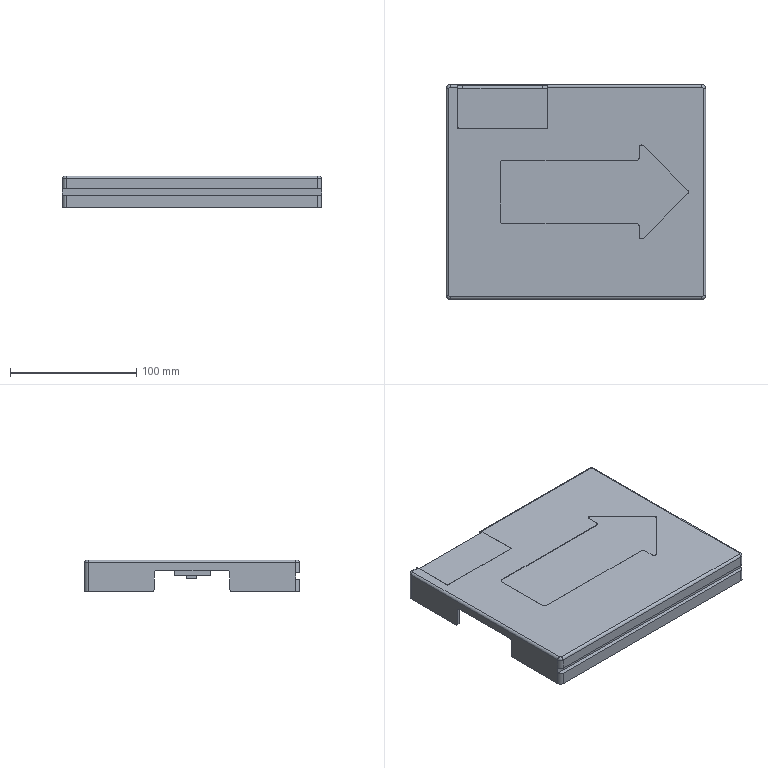NC program | NX | posted with a generic post | part box 205 x 170 x 25 mm
Lines 6527 to 7366 of 17262:
(CAVITY_MILL_1_COPY , TOOL : D4)
N13040 T17 M6
N13042 G54
N13044 G17 G0 G90 X-97.7 Y-73.808 B0. C0. S9500 M3
N13046 G43 Z30. H17
N13048 Z-0.4
N13050 G94 G1 X-98. Y-73.981 F1000.
N13052 G3 X-98.5 Y-74.847 R1.
N13054 G1 Y-76.999 F1600.
N13056 G3 X-97.494 Y-78. R1.
N13058 G1 X-95.347
N13060 G3 X-94.481 Y-77.5 R1.
N13062 G1 X-94.308 Y-77.2
N13064 G0 X-97.7 Y-73.808 Z-0.8
N13066 G1 X-98. Y-73.981 F1000.
N13068 G3 X-98.5 Y-74.847 R1.
N13070 G1 Y-76.999 F1600.
N13072 G3 X-97.494 Y-78. R1.
N13074 G1 X-95.347
N13076 G3 X-94.481 Y-77.5 R1.
N13078 G1 X-94.308 Y-77.2
N13080 G0 X-97.7 Y-73.808 Z-1.2
N13082 G1 X-98. Y-73.981 F1000.
N13084 G3 X-98.5 Y-74.847 R1.
N13086 G1 Y-76.999 F1600.
N13088 G3 X-97.494 Y-78. R1.
N13090 G1 X-95.347
N13092 G3 X-94.481 Y-77.5 R1.
N13094 G1 X-94.308 Y-77.2
N13096 G0 X-97.7 Y-73.808 Z-1.6
N13098 G1 X-98. Y-73.981 F1000.
N13100 G3 X-98.5 Y-74.847 R1.
N13102 G1 Y-76.999 F1600.
N13104 G3 X-97.494 Y-78. R1.
N13106 G1 X-95.347
N13108 G3 X-94.481 Y-77.5 R1.
N13110 G1 X-94.308 Y-77.2
N13112 G0 X-97.7 Y-73.808 Z-2.
N13114 G1 X-98. Y-73.981 F1000.
N13116 G3 X-98.5 Y-74.847 R1.
N13118 G1 Y-76.999 F1600.
N13120 G3 X-97.494 Y-78. R1.
N13122 G1 X-95.347
N13124 G3 X-94.481 Y-77.5 R1.
N13126 G1 X-94.308 Y-77.2
N13128 G0 X-97.7 Y-73.808 Z-2.4
N13130 G1 X-98. Y-73.981 F1000.
N13132 G3 X-98.5 Y-74.847 R1.
N13134 G1 Y-76.999 F1600.
N13136 G3 X-97.494 Y-78. R1.
N13138 G1 X-95.347
N13140 G3 X-94.481 Y-77.5 R1.
N13142 G1 X-94.308 Y-77.2
N13144 G0 X-97.7 Y-73.808 Z-2.8
N13146 G1 X-98. Y-73.981 F1000.
N13148 G3 X-98.5 Y-74.847 R1.
N13150 G1 Y-76.999 F1600.
N13152 G3 X-97.494 Y-78. R1.
N13154 G1 X-95.347
N13156 G3 X-94.481 Y-77.5 R1.
N13158 G1 X-94.308 Y-77.2
N13160 G0 X-97.7 Y-73.808 Z-3.2
N13162 G1 X-98. Y-73.981 F1000.
N13164 G3 X-98.5 Y-74.847 R1.
N13166 G1 Y-76.999 F1600.
N13168 G3 X-97.494 Y-78. R1.
N13170 G1 X-95.347
N13172 G3 X-94.481 Y-77.5 R1.
N13174 G1 X-94.308 Y-77.2
N13176 G0 X-97.7 Y-73.808 Z-3.6
N13178 G1 X-98. Y-73.981 F1000.
N13180 G3 X-98.5 Y-74.847 R1.
N13182 G1 Y-76.999 F1600.
N13184 G3 X-97.494 Y-78. R1.
N13186 G1 X-95.347
N13188 G3 X-94.481 Y-77.5 R1.
N13190 G1 X-94.308 Y-77.2
N13192 G0 X-97.7 Y-73.808 Z-4.
N13194 G1 X-98. Y-73.981 F1000.
N13196 G3 X-98.5 Y-74.847 R1.
N13198 G1 Y-76.999 F1600.
N13200 G3 X-97.494 Y-78. R1.
N13202 G1 X-95.347
N13204 G3 X-94.481 Y-77.5 R1.
N13206 G1 X-94.308 Y-77.2
N13208 G0 X-97.7 Y-73.808 Z-4.4
N13210 G1 X-98. Y-73.981 F1000.
N13212 G3 X-98.5 Y-74.847 R1.
N13214 G1 Y-76.999 F1600.
N13216 G3 X-97.494 Y-78. R1.
N13218 G1 X-95.347
N13220 G3 X-94.481 Y-77.5 R1.
N13222 G1 X-94.308 Y-77.2
N13224 G0 X-97.7 Y-73.808 Z-4.8
N13226 G1 X-98. Y-73.981 F1000.
N13228 G3 X-98.5 Y-74.847 R1.
N13230 G1 Y-76.999 F1600.
N13232 G3 X-97.494 Y-78. R1.
N13234 G1 X-95.347
N13236 G3 X-94.481 Y-77.5 R1.
N13238 G1 X-94.308 Y-77.2
N13240 G0 X-97.7 Y-73.808 Z-5.2
N13242 G1 X-98. Y-73.981 F1000.
N13244 G3 X-98.5 Y-74.847 R1.
N13246 G1 Y-76.999 F1600.
N13248 G3 X-97.494 Y-78. R1.
N13250 G1 X-95.347
N13252 G3 X-94.481 Y-77.5 R1.
N13254 G1 X-94.308 Y-77.2
N13256 G0 X-97.7 Y-73.808 Z-5.6
N13258 G1 X-98. Y-73.981 F1000.
N13260 G3 X-98.5 Y-74.847 R1.
N13262 G1 Y-76.999 F1600.
N13264 G3 X-97.494 Y-78. R1.
N13266 G1 X-95.347
N13268 G3 X-94.481 Y-77.5 R1.
N13270 G1 X-94.308 Y-77.2
N13272 G0 X-97.7 Y-73.808 Z-6.
N13274 G1 X-98. Y-73.981 F1000.
N13276 G3 X-98.5 Y-74.847 R1.
N13278 G1 Y-76.999 F1600.
N13280 G3 X-97.494 Y-78. R1.
N13282 G1 X-95.347
N13284 G3 X-94.481 Y-77.5 R1.
N13286 G1 X-94.308 Y-77.2
N13288 G0 X-97.7 Y-73.808 Z-6.4
N13290 G1 X-98. Y-73.981 F1000.
N13292 G3 X-98.5 Y-74.847 R1.
N13294 G1 Y-76.999 F1600.
N13296 G3 X-97.494 Y-78. R1.
N13298 G1 X-95.347
N13300 G3 X-94.481 Y-77.5 R1.
N13302 G1 X-94.308 Y-77.2
N13304 G0 X-97.7 Y-73.808 Z-6.8
N13306 G1 X-98. Y-73.981 F1000.
N13308 G3 X-98.5 Y-74.847 R1.
N13310 G1 Y-76.999 F1600.
N13312 G3 X-97.494 Y-78. R1.
N13314 G1 X-95.347
N13316 G3 X-94.481 Y-77.5 R1.
N13318 G1 X-94.308 Y-77.2
N13320 G0 X-97.7 Y-73.808 Z-7.2
N13322 G1 X-98. Y-73.981 F1000.
N13324 G3 X-98.5 Y-74.847 R1.
N13326 G1 Y-76.999 F1600.
N13328 G3 X-97.494 Y-78. R1.
N13330 G1 X-95.347
N13332 G3 X-94.481 Y-77.5 R1.
N13334 G1 X-94.308 Y-77.2
N13336 G0 X-97.7 Y-73.808 Z-7.6
N13338 G1 X-98. Y-73.981 F1000.
N13340 G3 X-98.5 Y-74.847 R1.
N13342 G1 Y-76.999 F1600.
N13344 G3 X-97.494 Y-78. R1.
N13346 G1 X-95.347
N13348 G3 X-94.481 Y-77.5 R1.
N13350 G1 X-94.308 Y-77.2
N13352 G0 X-97.7 Y-73.808 Z-8.
N13354 G1 X-98. Y-73.981 F1000.
N13356 G3 X-98.5 Y-74.847 R1.
N13358 G1 Y-76.999 F1600.
N13360 G3 X-97.494 Y-78. R1.
N13362 G1 X-95.347
N13364 G3 X-94.481 Y-77.5 R1.
N13366 G1 X-94.308 Y-77.2
N13368 G0 X-90.471 Y-72.752 Z-8.4
N13370 G1 X-90.719 Y-72.763 F1000.
N13372 G3 X-91.561 Y-73.302 R1.
N13374 G2 X-96.013 Y-76. R5. F1600.
N13376 G1 X-97.502
N13378 G3 X-98.5 Y-76.999 R1.
N13380 X-97.494 Y-78. R1.
N13382 G1 X-88.919
N13384 G3 X-88.053 Y-77.5 R1.
N13386 G1 X-87.88 Y-77.2
N13388 G0 X-90.471 Y-72.752 Z-8.8
N13390 G1 X-90.719 Y-72.763 F1000.
N13392 G3 X-91.561 Y-73.302 R1.
N13394 G2 X-96.013 Y-76. R5. F1600.
N13396 G1 X-97.502
N13398 G3 X-98.5 Y-76.999 R1.
N13400 X-97.494 Y-78. R1.
N13402 G1 X-88.919
N13404 G3 X-88.053 Y-77.5 R1.
N13406 G1 X-87.88 Y-77.2
N13408 G0 X-90.471 Y-72.752 Z-9.2
N13410 G1 X-90.719 Y-72.763 F1000.
N13412 G3 X-91.561 Y-73.302 R1.
N13414 G2 X-96.013 Y-76. R5. F1600.
N13416 G1 X-97.502
N13418 G3 X-98.5 Y-76.999 R1.
N13420 X-97.494 Y-78. R1.
N13422 G1 X-88.919
N13424 G3 X-88.053 Y-77.5 R1.
N13426 G1 X-87.88 Y-77.2
N13428 G0 X-90.471 Y-72.752 Z-9.6
N13430 G1 X-90.719 Y-72.763 F1000.
N13432 G3 X-91.561 Y-73.302 R1.
N13434 G2 X-96.013 Y-76. R5. F1600.
N13436 G1 X-97.502
N13438 G3 X-98.5 Y-76.999 R1.
N13440 X-97.494 Y-78. R1.
N13442 G1 X-88.919
N13444 G3 X-88.053 Y-77.5 R1.
N13446 G1 X-87.88 Y-77.2
N13448 G0 X-90.471 Y-72.752 Z-10.
N13450 G1 X-90.719 Y-72.763 F1000.
N13452 G3 X-91.561 Y-73.302 R1.
N13454 G2 X-96.013 Y-76. R5. F1600.
N13456 G1 X-97.502
N13458 G3 X-98.5 Y-76.999 R1.
N13460 X-97.494 Y-78. R1.
N13462 G1 X-88.919
N13464 G3 X-88.053 Y-77.5 R1.
N13466 G1 X-87.88 Y-77.2
N13468 G0 X-90.471 Y-72.752 Z-10.4
N13470 G1 X-90.719 Y-72.763 F1000.
N13472 G3 X-91.561 Y-73.302 R1.
N13474 G2 X-96.013 Y-76. R5. F1600.
N13476 G1 X-97.502
N13478 G3 X-98.5 Y-76.999 R1.
N13480 X-97.494 Y-78. R1.
N13482 G1 X-88.919
N13484 G3 X-88.053 Y-77.5 R1.
N13486 G1 X-87.88 Y-77.2
N13488 G0 X-90.471 Y-72.752 Z-10.8
N13490 G1 X-90.719 Y-72.763 F1000.
N13492 G3 X-91.561 Y-73.302 R1.
N13494 G2 X-96.013 Y-76. R5. F1600.
N13496 G1 X-97.502
N13498 G3 X-98.5 Y-76.999 R1.
N13500 X-97.494 Y-78. R1.
N13502 G1 X-88.919
N13504 G3 X-88.053 Y-77.5 R1.
N13506 G1 X-87.88 Y-77.2
N13508 G0 X-90.471 Y-72.752 Z-11.2
N13510 G1 X-90.719 Y-72.763 F1000.
N13512 G3 X-91.561 Y-73.302 R1.
N13514 G2 X-96.013 Y-76. R5. F1600.
N13516 G1 X-97.502
N13518 G3 X-98.5 Y-76.999 R1.
N13520 X-97.494 Y-78. R1.
N13522 G1 X-88.919
N13524 G3 X-88.053 Y-77.5 R1.
N13526 G1 X-87.88 Y-77.2
N13528 G0 X-90.471 Y-72.752 Z-11.6
N13530 G1 X-90.719 Y-72.763 F1000.
N13532 G3 X-91.561 Y-73.302 R1.
N13534 G2 X-96.013 Y-76. R5. F1600.
N13536 G1 X-97.502
N13538 G3 X-98.5 Y-76.999 R1.
N13540 X-97.494 Y-78. R1.
N13542 G1 X-88.919
N13544 G3 X-88.053 Y-77.5 R1.
N13546 G1 X-87.88 Y-77.2
N13548 G0 X-90.471 Y-72.752 Z-12.
N13550 G1 X-90.719 Y-72.763 F1000.
N13552 G3 X-91.561 Y-73.302 R1.
N13554 G2 X-96.013 Y-76. R5. F1600.
N13556 G1 X-97.502
N13558 G3 X-98.5 Y-76.999 R1.
N13560 X-97.494 Y-78. R1.
N13562 G1 X-88.919
N13564 G3 X-88.053 Y-77.5 R1.
N13566 G1 X-87.88 Y-77.2
N13568 G0 X-90.471 Y-72.752 Z-12.4
N13570 G1 X-90.719 Y-72.763 F1000.
N13572 G3 X-91.561 Y-73.302 R1.
N13574 G2 X-96.013 Y-76. R5. F1600.
N13576 G1 X-97.502
N13578 G3 X-98.5 Y-76.999 R1.
N13580 X-97.494 Y-78. R1.
N13582 G1 X-88.919
N13584 G3 X-88.053 Y-77.5 R1.
N13586 G1 X-87.88 Y-77.2
N13588 G0 X-90.471 Y-72.752 Z-12.8
N13590 G1 X-90.719 Y-72.763 F1000.
N13592 G3 X-91.561 Y-73.302 R1.
N13594 G2 X-96.013 Y-76. R5. F1600.
N13596 G1 X-97.502
N13598 G3 X-98.5 Y-76.999 R1.
N13600 X-97.494 Y-78. R1.
N13602 G1 X-88.919
N13604 G3 X-88.053 Y-77.5 R1.
N13606 G1 X-87.88 Y-77.2
N13608 G0 X-90.471 Y-72.752 Z-13.15
N13610 G1 X-90.719 Y-72.763 F1000.
N13612 G3 X-91.561 Y-73.302 R1.
N13614 G2 X-96.013 Y-76. R5. F1600.
N13616 G1 X-97.502
N13618 G3 X-98.5 Y-76.999 R1.
N13620 X-97.494 Y-78. R1.
N13622 G1 X-88.919
N13624 G3 X-88.053 Y-77.5 R1.
N13626 G1 X-87.88 Y-77.2
N13628 G0 X-90.471 Y-72.752 Z-13.5
N13630 G1 X-90.719 Y-72.763 F1000.
N13632 G3 X-91.561 Y-73.302 R1.
N13634 G2 X-96.013 Y-76. R5. F1600.
N13636 G1 X-97.502
N13638 G3 X-98.5 Y-76.999 R1.
N13640 X-97.494 Y-78. R1.
N13642 G1 X-88.919
N13644 G3 X-88.053 Y-77.5 R1.
N13646 G1 X-87.88 Y-77.2
N13648 G0 X-90.471 Y-72.752 Z-13.85
N13650 G1 X-90.719 Y-72.763 F1000.
N13652 G3 X-91.561 Y-73.302 R1.
N13654 G2 X-96.013 Y-76. R5. F1600.
N13656 G1 X-97.502
N13658 G3 X-98.5 Y-76.999 R1.
N13660 X-97.494 Y-78. R1.
N13662 G1 X-88.919
N13664 G3 X-88.053 Y-77.5 R1.
N13666 G1 X-87.88 Y-77.2
N13668 G0 X-90.471 Y-72.752 Z-14.2
N13670 G1 X-90.719 Y-72.763 F1000.
N13672 G3 X-91.561 Y-73.302 R1.
N13674 G2 X-96.013 Y-76. R5. F1600.
N13676 G1 X-97.502
N13678 G3 X-98.5 Y-76.999 R1.
N13680 X-97.494 Y-78. R1.
N13682 G1 X-88.919
N13684 G3 X-88.053 Y-77.5 R1.
N13686 G1 X-87.88 Y-77.2
N13688 G0 X-90.471 Y-72.752 Z-14.6
N13690 G1 X-90.719 Y-72.763 F1000.
N13692 G3 X-91.561 Y-73.302 R1.
N13694 G2 X-96.013 Y-76. R5. F1600.
N13696 G1 X-97.502
N13698 G3 X-98.5 Y-76.999 R1.
N13700 X-97.494 Y-78. R1.
N13702 G1 X-88.919
N13704 G3 X-88.053 Y-77.5 R1.
N13706 G1 X-87.88 Y-77.2
N13708 G0 X-90.471 Y-72.752 Z-15.
N13710 G1 X-90.719 Y-72.763 F1000.
N13712 G3 X-91.561 Y-73.302 R1.
N13714 G2 X-96.013 Y-76. R5. F1600.
N13716 G1 X-97.502
N13718 G3 X-98.5 Y-76.999 R1.
N13720 X-97.494 Y-78. R1.
N13722 G1 X-88.919
N13724 G3 X-88.053 Y-77.5 R1.
N13726 G1 X-87.88 Y-77.2
N13728 G0 X-90.471 Y-72.752 Z-15.4
N13730 G1 X-90.719 Y-72.763 F1000.
N13732 G3 X-91.561 Y-73.302 R1.
N13734 G2 X-96.013 Y-76. R5. F1600.
N13736 G1 X-97.502
N13738 G3 X-98.5 Y-76.999 R1.
N13740 X-97.494 Y-78. R1.
N13742 G1 X-88.919
N13744 G3 X-88.053 Y-77.5 R1.
N13746 G1 X-87.88 Y-77.2
N13748 G0 X-90.471 Y-72.752 Z-15.8
N13750 G1 X-90.719 Y-72.763 F1000.
N13752 G3 X-91.561 Y-73.302 R1.
N13754 G2 X-96.013 Y-76. R5. F1600.
N13756 G1 X-97.502
N13758 G3 X-98.5 Y-76.999 R1.
N13760 X-97.494 Y-78. R1.
N13762 G1 X-88.919
N13764 G3 X-88.053 Y-77.5 R1.
N13766 G1 X-87.88 Y-77.2
N13768 G0 X-90.471 Y-72.752 Z-16.2
N13770 G1 X-90.719 Y-72.763 F1000.
N13772 G3 X-91.561 Y-73.302 R1.
N13774 G2 X-96.013 Y-76. R5. F1600.
N13776 G1 X-97.502
N13778 G3 X-98.5 Y-76.999 R1.
N13780 X-97.494 Y-78. R1.
N13782 G1 X-88.919
N13784 G3 X-88.053 Y-77.5 R1.
N13786 G1 X-87.88 Y-77.2
N13788 G0 X-90.471 Y-72.752 Z-16.6
N13790 G1 X-90.719 Y-72.763 F1000.
N13792 G3 X-91.561 Y-73.302 R1.
N13794 G2 X-96.013 Y-76. R5. F1600.
N13796 G1 X-97.502
N13798 G3 X-98.5 Y-76.999 R1.
N13800 X-97.494 Y-78. R1.
N13802 G1 X-88.919
N13804 G3 X-88.053 Y-77.5 R1.
N13806 G1 X-87.88 Y-77.2
N13808 G0 X-90.471 Y-72.752 Z-17.
N13810 G1 X-90.719 Y-72.763 F1000.
N13812 G3 X-91.561 Y-73.302 R1.
N13814 G2 X-96.013 Y-76. R5. F1600.
N13816 G1 X-97.502
N13818 G3 X-98.5 Y-76.999 R1.
N13820 X-97.494 Y-78. R1.
N13822 G1 X-88.919
N13824 G3 X-88.053 Y-77.5 R1.
N13826 G1 X-87.88 Y-77.2
N13828 G0 X-90.471 Y-72.752 Z-17.385
N13830 G1 X-90.719 Y-72.763 F1000.
N13832 G3 X-91.561 Y-73.302 R1.
N13834 G2 X-96.013 Y-76. R5. F1600.
N13836 G1 X-97.502
N13838 G3 X-98.5 Y-76.999 R1.
N13840 X-97.494 Y-78. R1.
N13842 G1 X-88.919
N13844 G3 X-88.053 Y-77.5 R1.
N13846 G1 X-87.88 Y-77.2
N13848 G0 X-90.471 Y-72.752 Z-17.769
N13850 G1 X-90.719 Y-72.763 F1000.
N13852 G3 X-91.561 Y-73.302 R1.
N13854 G2 X-96.013 Y-76. R5. F1600.
N13856 G1 X-97.502
N13858 G3 X-98.5 Y-76.999 R1.
N13860 X-97.494 Y-78. R1.
N13862 G1 X-88.919
N13864 G3 X-88.053 Y-77.5 R1.
N13866 G1 X-87.88 Y-77.2
N13868 G0 X-90.471 Y-72.752 Z-18.154
N13870 G1 X-90.719 Y-72.763 F1000.
N13872 G3 X-91.561 Y-73.302 R1.
N13874 G2 X-96.013 Y-76. R5. F1600.
N13876 G1 X-97.502
N13878 G3 X-98.5 Y-76.999 R1.
N13880 X-97.494 Y-78. R1.
N13882 G1 X-88.919
N13884 G3 X-88.053 Y-77.5 R1.
N13886 G1 X-87.88 Y-77.2
N13888 G0 X-90.471 Y-72.752 Z-18.538
N13890 G1 X-90.719 Y-72.763 F1000.
N13892 G3 X-91.561 Y-73.302 R1.
N13894 G2 X-96.013 Y-76. R5. F1600.
N13896 G1 X-97.502
N13898 G3 X-98.5 Y-76.999 R1.
N13900 X-97.494 Y-78. R1.
N13902 G1 X-88.919
N13904 G3 X-88.053 Y-77.5 R1.
N13906 G1 X-87.88 Y-77.2
N13908 G0 X-90.471 Y-72.752 Z-18.923
N13910 G1 X-90.719 Y-72.763 F1000.
N13912 G3 X-91.561 Y-73.302 R1.
N13914 G2 X-96.013 Y-76. R5. F1600.
N13916 G1 X-97.502
N13918 G3 X-98.5 Y-76.999 R1.
N13920 X-97.494 Y-78. R1.
N13922 G1 X-88.919
N13924 G3 X-88.053 Y-77.5 R1.
N13926 G1 X-87.88 Y-77.2
N13928 G0 X-90.471 Y-72.752 Z-19.308
N13930 G1 X-90.719 Y-72.763 F1000.
N13932 G3 X-91.561 Y-73.302 R1.
N13934 G2 X-96.013 Y-76. R5. F1600.
N13936 G1 X-97.502
N13938 G3 X-98.5 Y-76.999 R1.
N13940 X-97.494 Y-78. R1.
N13942 G1 X-88.919
N13944 G3 X-88.053 Y-77.5 R1.
N13946 G1 X-87.88 Y-77.2
N13948 G0 X-90.471 Y-72.752 Z-19.692
N13950 G1 X-90.719 Y-72.763 F1000.
N13952 G3 X-91.561 Y-73.302 R1.
N13954 G2 X-96.013 Y-76. R5. F1600.
N13956 G1 X-97.502
N13958 G3 X-98.5 Y-76.999 R1.
N13960 X-97.494 Y-78. R1.
N13962 G1 X-88.919
N13964 G3 X-88.053 Y-77.5 R1.
N13966 G1 X-87.88 Y-77.2
N13968 G0 X-90.471 Y-72.752 Z-20.077
N13970 G1 X-90.719 Y-72.763 F1000.
N13972 G3 X-91.561 Y-73.302 R1.
N13974 G2 X-96.013 Y-76. R5. F1600.
N13976 G1 X-97.502
N13978 G3 X-98.5 Y-76.999 R1.
N13980 X-97.494 Y-78. R1.
N13982 G1 X-88.919
N13984 G3 X-88.053 Y-77.5 R1.
N13986 G1 X-87.88 Y-77.2
N13988 G0 X-90.471 Y-72.752 Z-20.462
N13990 G1 X-90.719 Y-72.763 F1000.
N13992 G3 X-91.561 Y-73.302 R1.
N13994 G2 X-96.013 Y-76. R5. F1600.
N13996 G1 X-97.502
N13998 G3 X-98.5 Y-76.999 R1.
N14000 X-97.494 Y-78. R1.
N14002 G1 X-88.919
N14004 G3 X-88.053 Y-77.5 R1.
N14006 G1 X-87.88 Y-77.2
N14008 G0 X-90.471 Y-72.752 Z-20.846
N14010 G1 X-90.719 Y-72.763 F1000.
N14012 G3 X-91.561 Y-73.302 R1.
N14014 G2 X-96.013 Y-76. R5. F1600.
N14016 G1 X-97.502
N14018 G3 X-98.5 Y-76.999 R1.
N14020 X-97.494 Y-78. R1.
N14022 G1 X-88.919
N14024 G3 X-88.053 Y-77.5 R1.
N14026 G1 X-87.88 Y-77.2
N14028 G0 X-90.471 Y-72.752 Z-21.231
N14030 G1 X-90.719 Y-72.763 F1000.
N14032 G3 X-91.561 Y-73.302 R1.
N14034 G2 X-96.013 Y-76. R5. F1600.
N14036 G1 X-97.502
N14038 G3 X-98.5 Y-76.999 R1.
N14040 X-97.494 Y-78. R1.
N14042 G1 X-88.919
N14044 G3 X-88.053 Y-77.5 R1.
N14046 G1 X-87.88 Y-77.2
N14048 G0 X-90.471 Y-72.752 Z-21.615
N14050 G1 X-90.719 Y-72.763 F1000.
N14052 G3 X-91.561 Y-73.302 R1.
N14054 G2 X-96.013 Y-76. R5. F1600.
N14056 G1 X-97.502
N14058 G3 X-98.5 Y-76.999 R1.
N14060 X-97.494 Y-78. R1.
N14062 G1 X-88.919
N14064 G3 X-88.053 Y-77.5 R1.
N14066 G1 X-87.88 Y-77.2
N14068 G0 X-90.471 Y-72.752 Z-22.
N14070 G1 X-90.719 Y-72.763 F1000.
N14072 G3 X-91.561 Y-73.302 R1.
N14074 G2 X-96.013 Y-76. R5. F1600.
N14076 G1 X-97.502
N14078 G3 X-98.5 Y-76.999 R1.
N14080 X-97.494 Y-78. R1.
N14082 G1 X-88.919
N14084 G3 X-88.053 Y-77.5 R1.
N14086 G1 X-87.88 Y-77.2
N14088 G0 Z30.
N14090 X-97.7 Y-61.823
N14092 Z-8.4
N14094 G1 X-98. Y-61.997 F1000.
N14096 G3 X-98.5 Y-62.863 R1.
N14098 G1 Y-64.998 F1600.
N14100 G3 X-97.494 Y-66. R1.
N14102 G1 X-96.
N14104 G2 X-95.462 Y-66.029 R5.
N14106 G3 X-94.548 Y-65.625 R1.
N14108 G1 X-94.401 Y-65.425
N14110 G0 X-97.7 Y-61.823 Z-8.8
N14112 G1 X-98. Y-61.997 F1000.
N14114 G3 X-98.5 Y-62.863 R1.
N14116 G1 Y-64.998 F1600.
N14118 G3 X-97.494 Y-66. R1.
N14120 G1 X-96.001
N14122 G2 X-95.463 Y-66.029 R5.
N14124 G3 X-94.548 Y-65.625 R1.
N14126 G1 X-94.401 Y-65.425
N14128 G0 X-97.7 Y-61.823 Z-9.2
N14130 G1 X-98. Y-61.997 F1000.
N14132 G3 X-98.5 Y-62.863 R1.
N14134 G1 Y-64.998 F1600.
N14136 G3 X-97.494 Y-66. R1.
N14138 G1 X-96.001
N14140 G2 X-95.463 Y-66.029 R5.
N14142 G3 X-94.548 Y-65.625 R1.
N14144 G1 X-94.401 Y-65.425
N14146 G0 X-97.7 Y-61.823 Z-9.6
N14148 G1 X-98. Y-61.997 F1000.
N14150 G3 X-98.5 Y-62.863 R1.
N14152 G1 Y-64.998 F1600.
N14154 G3 X-97.494 Y-66. R1.
N14156 G1 X-96.001
N14158 G2 X-95.463 Y-66.029 R5.
N14160 G3 X-94.548 Y-65.625 R1.
N14162 G1 X-94.401 Y-65.425
N14164 G0 X-97.7 Y-61.823 Z-10.
N14166 G1 X-98. Y-61.997 F1000.
N14168 G3 X-98.5 Y-62.863 R1.
N14170 G1 Y-64.998 F1600.
N14172 G3 X-97.494 Y-66. R1.
N14174 G1 X-96.001
N14176 G2 X-95.463 Y-66.029 R5.
N14178 G3 X-94.548 Y-65.625 R1.
N14180 G1 X-94.401 Y-65.425
N14182 G0 X-97.7 Y-61.823 Z-10.4
N14184 G1 X-98. Y-61.997 F1000.
N14186 G3 X-98.5 Y-62.863 R1.
N14188 G1 Y-64.998 F1600.
N14190 G3 X-97.494 Y-66. R1.
N14192 G1 X-96.001
N14194 G2 X-95.463 Y-66.029 R5.
N14196 G3 X-94.548 Y-65.625 R1.
N14198 G1 X-94.401 Y-65.425
N14200 G0 X-97.7 Y-61.823 Z-10.8
N14202 G1 X-98. Y-61.997 F1000.
N14204 G3 X-98.5 Y-62.863 R1.
N14206 G1 Y-64.998 F1600.
N14208 G3 X-97.494 Y-66. R1.
N14210 G1 X-96.001
N14212 G2 X-95.463 Y-66.029 R5.
N14214 G3 X-94.548 Y-65.625 R1.
N14216 G1 X-94.401 Y-65.425
N14218 G0 X-97.7 Y-61.823 Z-11.2
N14220 G1 X-98. Y-61.997 F1000.
N14222 G3 X-98.5 Y-62.863 R1.
N14224 G1 Y-64.998 F1600.
N14226 G3 X-97.494 Y-66. R1.
N14228 G1 X-96.001
N14230 G2 X-95.463 Y-66.029 R5.
N14232 G3 X-94.548 Y-65.625 R1.
N14234 G1 X-94.401 Y-65.425
N14236 G0 X-97.7 Y-61.823 Z-11.6
N14238 G1 X-98. Y-61.997 F1000.
N14240 G3 X-98.5 Y-62.863 R1.
N14242 G1 Y-64.998 F1600.
N14244 G3 X-97.494 Y-66. R1.
N14246 G1 X-96.001
N14248 G2 X-95.463 Y-66.029 R5.
N14250 G3 X-94.548 Y-65.625 R1.
N14252 G1 X-94.401 Y-65.425
N14254 G0 X-97.7 Y-61.823 Z-12.
N14256 G1 X-98. Y-61.997 F1000.
N14258 G3 X-98.5 Y-62.863 R1.
N14260 G1 Y-64.998 F1600.
N14262 G3 X-97.494 Y-66. R1.
N14264 G1 X-96.001
N14266 G2 X-95.463 Y-66.029 R5.
N14268 G3 X-94.548 Y-65.625 R1.
N14270 G1 X-94.401 Y-65.425
N14272 G0 X-97.7 Y-61.823 Z-12.4
N14274 G1 X-98. Y-61.997 F1000.
N14276 G3 X-98.5 Y-62.863 R1.
N14278 G1 Y-64.998 F1600.
N14280 G3 X-97.494 Y-66. R1.
N14282 G1 X-96.001
N14284 G2 X-95.463 Y-66.029 R5.
N14286 G3 X-94.548 Y-65.625 R1.
N14288 G1 X-94.401 Y-65.425
N14290 G0 X-97.7 Y-61.823 Z-12.8
N14292 G1 X-98. Y-61.997 F1000.
N14294 G3 X-98.5 Y-62.863 R1.
N14296 G1 Y-64.998 F1600.
N14298 G3 X-97.494 Y-66. R1.
N14300 G1 X-96.001
N14302 G2 X-95.463 Y-66.029 R5.
N14304 G3 X-94.548 Y-65.625 R1.
N14306 G1 X-94.401 Y-65.425
N14308 G0 X-97.7 Y-61.823 Z-13.15
N14310 G1 X-98. Y-61.997 F1000.
N14312 G3 X-98.5 Y-62.863 R1.
N14314 G1 Y-64.998 F1600.
N14316 G3 X-97.494 Y-66. R1.
N14318 G1 X-96.001
N14320 G2 X-95.463 Y-66.029 R5.
N14322 G3 X-94.548 Y-65.625 R1.
N14324 G1 X-94.401 Y-65.425
N14326 G0 X-97.7 Y-61.823 Z-13.5
N14328 G1 X-98. Y-61.997 F1000.
N14330 G3 X-98.5 Y-62.863 R1.
N14332 G1 Y-64.998 F1600.
N14334 G3 X-97.494 Y-66. R1.
N14336 G1 X-96.001
N14338 G2 X-95.463 Y-66.029 R5.
N14340 G3 X-94.548 Y-65.625 R1.
N14342 G1 X-94.401 Y-65.425
N14344 G0 X-97.7 Y-61.823 Z-13.85
N14346 G1 X-98. Y-61.997 F1000.
N14348 G3 X-98.5 Y-62.863 R1.
N14350 G1 Y-64.998 F1600.
N14352 G3 X-97.494 Y-66. R1.
N14354 G1 X-96.001
N14356 G2 X-95.463 Y-66.029 R5.
N14358 G3 X-94.548 Y-65.625 R1.
N14360 G1 X-94.401 Y-65.425
N14362 G0 X-97.7 Y-61.823 Z-14.2
N14364 G1 X-98. Y-61.997 F1000.
N14366 G3 X-98.5 Y-62.863 R1.
N14368 G1 Y-64.998 F1600.
N14370 G3 X-97.494 Y-66. R1.
N14372 G1 X-96.001
N14374 G2 X-95.463 Y-66.029 R5.
N14376 G3 X-94.548 Y-65.625 R1.
N14378 G1 X-94.401 Y-65.425
N14380 G0 X-97.7 Y-61.823 Z-14.6
N14382 G1 X-98. Y-61.997 F1000.
N14384 G3 X-98.5 Y-62.863 R1.
N14386 G1 Y-64.998 F1600.
N14388 G3 X-97.494 Y-66. R1.
N14390 G1 X-96.001
N14392 G2 X-95.463 Y-66.029 R5.
N14394 G3 X-94.548 Y-65.625 R1.
N14396 G1 X-94.401 Y-65.425
N14398 G0 X-97.7 Y-61.823 Z-15.
N14400 G1 X-98. Y-61.997 F1000.
N14402 G3 X-98.5 Y-62.863 R1.
N14404 G1 Y-64.998 F1600.
N14406 G3 X-97.494 Y-66. R1.
N14408 G1 X-96.001
N14410 G2 X-95.463 Y-66.029 R5.
N14412 G3 X-94.548 Y-65.625 R1.
N14414 G1 X-94.401 Y-65.425
N14416 G0 X-97.7 Y-61.823 Z-15.4
N14418 G1 X-98. Y-61.997 F1000.
N14420 G3 X-98.5 Y-62.863 R1.
N14422 G1 Y-64.998 F1600.
N14424 G3 X-97.494 Y-66. R1.
N14426 G1 X-96.001
N14428 G2 X-95.463 Y-66.029 R5.
N14430 G3 X-94.548 Y-65.625 R1.
N14432 G1 X-94.401 Y-65.425
N14434 G0 X-97.7 Y-61.823 Z-15.8
N14436 G1 X-98. Y-61.997 F1000.
N14438 G3 X-98.5 Y-62.863 R1.
N14440 G1 Y-64.998 F1600.
N14442 G3 X-97.494 Y-66. R1.
N14444 G1 X-96.001
N14446 G2 X-95.463 Y-66.029 R5.
N14448 G3 X-94.548 Y-65.625 R1.
N14450 G1 X-94.401 Y-65.425
N14452 G0 X-97.7 Y-61.823 Z-16.2
N14454 G1 X-98. Y-61.997 F1000.
N14456 G3 X-98.5 Y-62.863 R1.
N14458 G1 Y-64.998 F1600.
N14460 G3 X-97.494 Y-66. R1.
N14462 G1 X-96.001
N14464 G2 X-95.463 Y-66.029 R5.
N14466 G3 X-94.548 Y-65.625 R1.
N14468 G1 X-94.401 Y-65.425
N14470 G0 X-97.7 Y-61.823 Z-16.6
N14472 G1 X-98. Y-61.997 F1000.
N14474 G3 X-98.5 Y-62.863 R1.
N14476 G1 Y-64.998 F1600.
N14478 G3 X-97.494 Y-66. R1.
N14480 G1 X-96.001
N14482 G2 X-95.463 Y-66.029 R5.
N14484 G3 X-94.548 Y-65.625 R1.
N14486 G1 X-94.401 Y-65.425
N14488 G0 X-97.7 Y-61.823 Z-17.
N14490 G1 X-98. Y-61.997 F1000.
N14492 G3 X-98.5 Y-62.863 R1.
N14494 G1 Y-64.998 F1600.
N14496 G3 X-97.494 Y-66. R1.
N14498 G1 X-96.001
N14500 G2 X-95.463 Y-66.029 R5.
N14502 G3 X-94.548 Y-65.625 R1.
N14504 G1 X-94.401 Y-65.425
N14506 G0 X-97.7 Y-61.823 Z-17.385
N14508 G1 X-98. Y-61.997 F1000.
N14510 G3 X-98.5 Y-62.863 R1.
N14512 G1 Y-64.998 F1600.
N14514 G3 X-97.494 Y-66. R1.
N14516 G1 X-96.001
N14518 G2 X-95.463 Y-66.029 R5.
N14520 G3 X-94.548 Y-65.625 R1.
N14522 G1 X-94.401 Y-65.425
N14524 G0 X-97.7 Y-61.823 Z-17.769
N14526 G1 X-98. Y-61.997 F1000.
N14528 G3 X-98.5 Y-62.863 R1.
N14530 G1 Y-64.998 F1600.
N14532 G3 X-97.494 Y-66. R1.
N14534 G1 X-96.001
N14536 G2 X-95.463 Y-66.029 R5.
N14538 G3 X-94.548 Y-65.625 R1.
N14540 G1 X-94.401 Y-65.425
N14542 G0 X-97.7 Y-61.823 Z-18.154
N14544 G1 X-98. Y-61.997 F1000.
N14546 G3 X-98.5 Y-62.863 R1.
N14548 G1 Y-64.998 F1600.
N14550 G3 X-97.494 Y-66. R1.
N14552 G1 X-96.001
N14554 G2 X-95.463 Y-66.029 R5.
N14556 G3 X-94.548 Y-65.625 R1.
N14558 G1 X-94.401 Y-65.425
N14560 G0 X-97.7 Y-61.823 Z-18.538
N14562 G1 X-98. Y-61.997 F1000.
N14564 G3 X-98.5 Y-62.863 R1.
N14566 G1 Y-64.998 F1600.
N14568 G3 X-97.494 Y-66. R1.
N14570 G1 X-96.001
N14572 G2 X-95.463 Y-66.029 R5.
N14574 G3 X-94.548 Y-65.625 R1.
N14576 G1 X-94.401 Y-65.425
N14578 G0 X-97.7 Y-61.823 Z-18.923
N14580 G1 X-98. Y-61.997 F1000.
N14582 G3 X-98.5 Y-62.863 R1.
N14584 G1 Y-64.998 F1600.
N14586 G3 X-97.494 Y-66. R1.
N14588 G1 X-96.001
N14590 G2 X-95.463 Y-66.029 R5.
N14592 G3 X-94.548 Y-65.625 R1.
N14594 G1 X-94.401 Y-65.425
N14596 G0 X-97.7 Y-61.823 Z-19.308
N14598 G1 X-98. Y-61.997 F1000.
N14600 G3 X-98.5 Y-62.863 R1.
N14602 G1 Y-64.998 F1600.
N14604 G3 X-97.494 Y-66. R1.
N14606 G1 X-96.001
N14608 G2 X-95.463 Y-66.029 R5.
N14610 G3 X-94.548 Y-65.625 R1.
N14612 G1 X-94.401 Y-65.425
N14614 G0 X-97.7 Y-61.823 Z-19.692
N14616 G1 X-98. Y-61.997 F1000.
N14618 G3 X-98.5 Y-62.863 R1.
N14620 G1 Y-64.998 F1600.
N14622 G3 X-97.494 Y-66. R1.
N14624 G1 X-96.001
N14626 G2 X-95.463 Y-66.029 R5.
N14628 G3 X-94.548 Y-65.625 R1.
N14630 G1 X-94.401 Y-65.425
N14632 G0 X-97.7 Y-61.823 Z-20.077
N14634 G1 X-98. Y-61.997 F1000.
N14636 G3 X-98.5 Y-62.863 R1.
N14638 G1 Y-64.998 F1600.
N14640 G3 X-97.494 Y-66. R1.
N14642 G1 X-96.001
N14644 G2 X-95.463 Y-66.029 R5.
N14646 G3 X-94.548 Y-65.625 R1.
N14648 G1 X-94.401 Y-65.425
N14650 G0 X-97.7 Y-61.823 Z-20.462
N14652 G1 X-98. Y-61.997 F1000.
N14654 G3 X-98.5 Y-62.863 R1.
N14656 G1 Y-64.998 F1600.
N14658 G3 X-97.494 Y-66. R1.
N14660 G1 X-96.001
N14662 G2 X-95.463 Y-66.029 R5.
N14664 G3 X-94.548 Y-65.625 R1.
N14666 G1 X-94.401 Y-65.425
N14668 G0 X-97.7 Y-61.823 Z-20.846
N14670 G1 X-98. Y-61.997 F1000.
N14672 G3 X-98.5 Y-62.863 R1.
N14674 G1 Y-64.998 F1600.
N14676 G3 X-97.494 Y-66. R1.
N14678 G1 X-96.001
N14680 G2 X-95.463 Y-66.029 R5.
N14682 G3 X-94.548 Y-65.625 R1.
N14684 G1 X-94.401 Y-65.425
N14686 G0 X-97.7 Y-61.823 Z-21.231
N14688 G1 X-98. Y-61.997 F1000.
N14690 G3 X-98.5 Y-62.863 R1.
N14692 G1 Y-64.998 F1600.
N14694 G3 X-97.494 Y-66. R1.
N14696 G1 X-96.001
N14698 G2 X-95.463 Y-66.029 R5.
N14700 G3 X-94.548 Y-65.625 R1.
N14702 G1 X-94.401 Y-65.425
N14704 G0 X-97.7 Y-61.823 Z-21.615
N14706 G1 X-98. Y-61.997 F1000.
N14708 G3 X-98.5 Y-62.863 R1.
N14710 G1 Y-64.998 F1600.
N14712 G3 X-97.494 Y-66. R1.